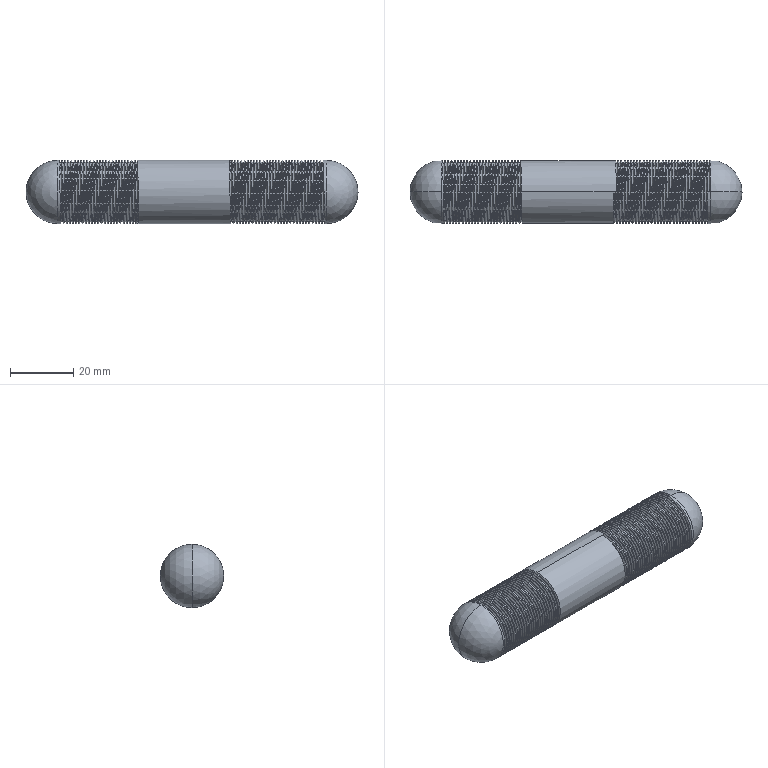Part | SolidWorks | features SweepThread 2, Fillet 1, RevolutionThin 1 | 1 solid | 126 faces | box 105 x 20 x 20 mm | volume 30081 mm3 | cylinder 112 | spline 6 | sphere 4 | plane 4 | commonest cylinder face diameters 20 x112